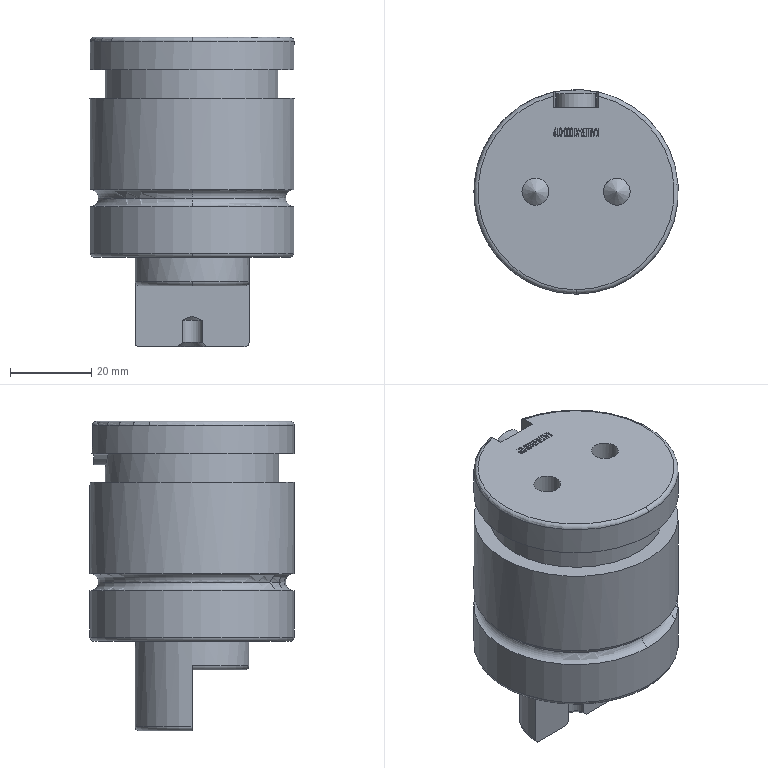Part | STEP file | 1_id1410_x_t | 1 solid | 183 faces | box 50.2 x 50.2 x 76 mm | volume 109766 mm3 | plane 130 | other 23 | torus 12 | cylinder 12 | cone 6 | commonest cylinder face diameters 50.2 x3 4.9 x2 6.6 x2 9.5 x2 11 x1 28 x1